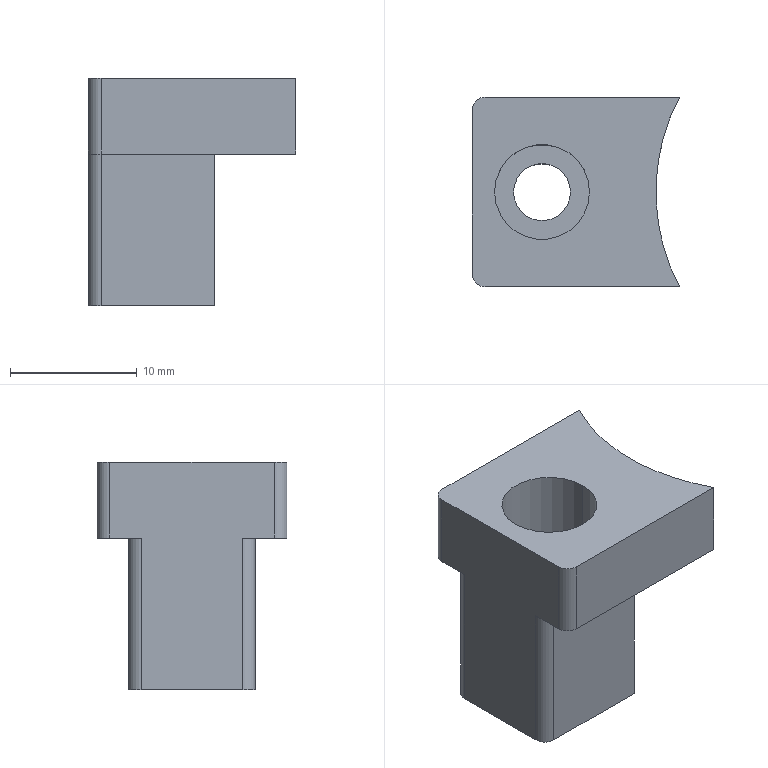Part | SolidWorks | features ICE 3, Fillet 2, Extrusion 1, HoleWzd 1, MirrorPattern 1 | 1 solid | 19 faces | box 16.367 x 15 x 18 mm | volume 2039 mm3 | plane 10 | cylinder 9 | commonest cylinder face diameters 2 x4 4.5 x2 7.5 x2 32 x1
STEP:
#1=CARTESIAN_POINT('',(-6.5,0.,10.));
#2=VERTEX_POINT('',#1);
#3=CARTESIAN_POINT('',(1.,0.,10.));
#4=VERTEX_POINT('',#3);
#5=CARTESIAN_POINT('',(-2.75,0.,10.));
#6=DIRECTION('',(0.,0.,1.));
#7=DIRECTION('',(1.,0.,0.));
#8=AXIS2_PLACEMENT_3D('',#5,#6,#7);
#9=CIRCLE('',#8,3.75);
#10=EDGE_CURVE('',#2,#4,#9,.T.);
#11=ORIENTED_EDGE('',*,*,#10,.F.);
#12=CARTESIAN_POINT('',(-6.5,0.,18.));
#13=VERTEX_POINT('',#12);
#14=CARTESIAN_POINT('',(-6.5,0.,18.));
#15=DIRECTION('',(0.,0.,1.));
#16=VECTOR('',#15,1000.);
#17=LINE('',#14,#16);
#18=EDGE_CURVE('',#2,#13,#17,.T.);
#19=ORIENTED_EDGE('',*,*,#18,.T.);
#20=CARTESIAN_POINT('',(1.,0.,18.));
#21=VERTEX_POINT('',#20);
#22=CARTESIAN_POINT('',(-2.75,0.,18.));
#23=DIRECTION('',(0.,0.,1.));
#24=DIRECTION('',(1.,0.,0.));
#25=AXIS2_PLACEMENT_3D('',#22,#23,#24);
#26=CIRCLE('',#25,3.75);
#27=EDGE_CURVE('',#13,#21,#26,.T.);
#28=ORIENTED_EDGE('',*,*,#27,.T.);
#29=CARTESIAN_POINT('',(1.,0.,18.));
#30=DIRECTION('',(0.,0.,1.));
#31=VECTOR('',#30,1000.);
#32=LINE('',#29,#31);
#33=EDGE_CURVE('',#4,#21,#32,.T.);
#34=ORIENTED_EDGE('',*,*,#33,.F.);
#35=EDGE_LOOP('',(#11,#19,#28,#34));
#36=FACE_OUTER_BOUND('',#35,.T.);
#37=CARTESIAN_POINT('',(-2.75,0.,18.));
#38=DIRECTION('',(0.,0.,1.));
#39=DIRECTION('',(1.,0.,0.));
#40=AXIS2_PLACEMENT_3D('',#37,#38,#39);
#41=CYLINDRICAL_SURFACE('',#40,3.75);
#42=ADVANCED_FACE('',(#36),#41,.F.);
#43=CARTESIAN_POINT('',(-5.,0.,0.));
#44=VERTEX_POINT('',#43);
#45=CARTESIAN_POINT('',(-0.5,0.,0.));
#46=VERTEX_POINT('',#45);
#47=CARTESIAN_POINT('',(-2.75,0.,0.));
#48=DIRECTION('',(0.,0.,1.));
#49=DIRECTION('',(1.,0.,0.));
#50=AXIS2_PLACEMENT_3D('',#47,#48,#49);
#51=CIRCLE('',#50,2.25);
#52=EDGE_CURVE('',#44,#46,#51,.T.);
#53=ORIENTED_EDGE('',*,*,#52,.F.);
#54=CARTESIAN_POINT('',(-5.,0.,10.));
#55=VERTEX_POINT('',#54);
#56=CARTESIAN_POINT('',(-5.,0.,18.));
#57=DIRECTION('',(0.,0.,1.));
#58=VECTOR('',#57,1000.);
#59=LINE('',#56,#58);
#60=EDGE_CURVE('',#44,#55,#59,.T.);
#61=ORIENTED_EDGE('',*,*,#60,.T.);
#62=CARTESIAN_POINT('',(-0.5,0.,10.));
#63=VERTEX_POINT('',#62);
#64=CARTESIAN_POINT('',(-2.75,0.,10.));
#65=DIRECTION('',(0.,0.,1.));
#66=DIRECTION('',(1.,0.,0.));
#67=AXIS2_PLACEMENT_3D('',#64,#65,#66);
#68=CIRCLE('',#67,2.25);
#69=EDGE_CURVE('',#55,#63,#68,.T.);
#70=ORIENTED_EDGE('',*,*,#69,.T.);
#71=CARTESIAN_POINT('',(-0.5,0.,18.));
#72=DIRECTION('',(0.,0.,1.));
#73=VECTOR('',#72,1000.);
#74=LINE('',#71,#73);
#75=EDGE_CURVE('',#46,#63,#74,.T.);
#76=ORIENTED_EDGE('',*,*,#75,.F.);
#77=EDGE_LOOP('',(#53,#61,#70,#76));
#78=FACE_OUTER_BOUND('',#77,.T.);
#79=CARTESIAN_POINT('',(-2.75,0.,18.));
#80=DIRECTION('',(0.,0.,1.));
#81=DIRECTION('',(1.,0.,0.));
#82=AXIS2_PLACEMENT_3D('',#79,#80,#81);
#83=CYLINDRICAL_SURFACE('',#82,2.25);
#84=ADVANCED_FACE('',(#78),#83,.F.);
#85=CARTESIAN_POINT('',(-7.25,7.5,12.));
#86=VERTEX_POINT('',#85);
#87=CARTESIAN_POINT('',(8.117,7.5,12.));
#88=VERTEX_POINT('',#87);
#89=CARTESIAN_POINT('',(1.75,7.5,12.));
#90=DIRECTION('',(1.,0.,0.));
#91=VECTOR('',#90,1000.);
#92=LINE('',#89,#91);
#93=EDGE_CURVE('',#86,#88,#92,.T.);
#94=ORIENTED_EDGE('',*,*,#93,.F.);
#95=CARTESIAN_POINT('',(-7.25,7.5,18.));
#96=VERTEX_POINT('',#95);
#97=CARTESIAN_POINT('',(-7.25,7.5,18.));
#98=DIRECTION('',(0.,0.,1.));
#99=VECTOR('',#98,1000.);
#100=LINE('',#97,#99);
#101=EDGE_CURVE('',#86,#96,#100,.T.);
#102=ORIENTED_EDGE('',*,*,#101,.T.);
#103=CARTESIAN_POINT('',(8.117,7.5,18.));
#104=VERTEX_POINT('',#103);
#105=CARTESIAN_POINT('',(-8.25,7.5,18.));
#106=DIRECTION('',(-1.,0.,0.));
#107=VECTOR('',#106,1000.);
#108=LINE('',#105,#107);
#109=EDGE_CURVE('',#104,#96,#108,.T.);
#110=ORIENTED_EDGE('',*,*,#109,.F.);
#111=CARTESIAN_POINT('',(8.117,7.5,0.));
#112=DIRECTION('',(0.,0.,-1.));
#113=VECTOR('',#112,1000.);
#114=LINE('',#111,#113);
#115=EDGE_CURVE('',#104,#88,#114,.T.);
#116=ORIENTED_EDGE('',*,*,#115,.T.);
#117=EDGE_LOOP('',(#94,#102,#110,#116));
#118=FACE_OUTER_BOUND('',#117,.T.);
#119=CARTESIAN_POINT('',(-8.25,7.5,18.));
#120=DIRECTION('',(0.,-1.,0.));
#121=DIRECTION('',(0.,0.,-1.));
#122=AXIS2_PLACEMENT_3D('',#119,#120,#121);
#123=PLANE('',#122);
#124=ADVANCED_FACE('',(#118),#123,.F.);
#125=CARTESIAN_POINT('',(-8.25,4.,12.));
#126=VERTEX_POINT('',#125);
#127=CARTESIAN_POINT('',(-8.25,6.5,12.));
#128=VERTEX_POINT('',#127);
#129=CARTESIAN_POINT('',(-8.25,5.,12.));
#130=DIRECTION('',(0.,1.,0.));
#131=VECTOR('',#130,1000.);
#132=LINE('',#129,#131);
#133=EDGE_CURVE('',#126,#128,#132,.T.);
#134=ORIENTED_EDGE('',*,*,#133,.F.);
#135=CARTESIAN_POINT('',(-8.25,4.,0.));
#136=VERTEX_POINT('',#135);
#137=CARTESIAN_POINT('',(-8.25,4.,18.));
#138=DIRECTION('',(0.,0.,-1.));
#139=VECTOR('',#138,1000.);
#140=LINE('',#137,#139);
#141=EDGE_CURVE('',#126,#136,#140,.T.);
#142=ORIENTED_EDGE('',*,*,#141,.T.);
#143=CARTESIAN_POINT('',(-8.25,-4.,0.));
#144=VERTEX_POINT('',#143);
#145=CARTESIAN_POINT('',(-8.25,7.5,0.));
#146=DIRECTION('',(0.,-1.,0.));
#147=VECTOR('',#146,1000.);
#148=LINE('',#145,#147);
#149=EDGE_CURVE('',#136,#144,#148,.T.);
#150=ORIENTED_EDGE('',*,*,#149,.T.);
#151=CARTESIAN_POINT('',(-8.25,-4.,12.));
#152=VERTEX_POINT('',#151);
#153=CARTESIAN_POINT('',(-8.25,-4.,18.));
#154=DIRECTION('',(0.,0.,1.));
#155=VECTOR('',#154,1000.);
#156=LINE('',#153,#155);
#157=EDGE_CURVE('',#144,#152,#156,.T.);
#158=ORIENTED_EDGE('',*,*,#157,.T.);
#159=CARTESIAN_POINT('',(-8.25,-6.5,12.));
#160=VERTEX_POINT('',#159);
#161=CARTESIAN_POINT('',(-8.25,-5.,12.));
#162=DIRECTION('',(0.,-1.,0.));
#163=VECTOR('',#162,1000.);
#164=LINE('',#161,#163);
#165=EDGE_CURVE('',#152,#160,#164,.T.);
#166=ORIENTED_EDGE('',*,*,#165,.T.);
#167=CARTESIAN_POINT('',(-8.25,-6.5,18.));
#168=VERTEX_POINT('',#167);
#169=CARTESIAN_POINT('',(-8.25,-6.5,18.));
#170=DIRECTION('',(0.,0.,1.));
#171=VECTOR('',#170,1000.);
#172=LINE('',#169,#171);
#173=EDGE_CURVE('',#160,#168,#172,.T.);
#174=ORIENTED_EDGE('',*,*,#173,.T.);
#175=CARTESIAN_POINT('',(-8.25,6.5,18.));
#176=VERTEX_POINT('',#175);
#177=CARTESIAN_POINT('',(-8.25,7.5,18.));
#178=DIRECTION('',(0.,-1.,0.));
#179=VECTOR('',#178,1000.);
#180=LINE('',#177,#179);
#181=EDGE_CURVE('',#176,#168,#180,.T.);
#182=ORIENTED_EDGE('',*,*,#181,.F.);
#183=CARTESIAN_POINT('',(-8.25,6.5,18.));
#184=DIRECTION('',(0.,0.,-1.));
#185=VECTOR('',#184,1000.);
#186=LINE('',#183,#185);
#187=EDGE_CURVE('',#176,#128,#186,.T.);
#188=ORIENTED_EDGE('',*,*,#187,.T.);
#189=EDGE_LOOP('',(#134,#142,#150,#158,#166,#174,#182,#188));
#190=FACE_OUTER_BOUND('',#189,.T.);
#191=CARTESIAN_POINT('',(-8.25,7.5,18.));
#192=DIRECTION('',(1.,0.,0.));
#193=DIRECTION('',(0.,1.,0.));
#194=AXIS2_PLACEMENT_3D('',#191,#192,#193);
#195=PLANE('',#194);
#196=ADVANCED_FACE('',(#190),#195,.F.);
#197=ORIENTED_EDGE('',*,*,#101,.F.);
#198=CARTESIAN_POINT('',(-7.25,6.5,12.));
#199=DIRECTION('',(0.,0.,1.));
#200=DIRECTION('',(-1.,0.,0.));
#201=AXIS2_PLACEMENT_3D('',#198,#199,#200);
#202=CIRCLE('',#201,1.);
#203=EDGE_CURVE('',#86,#128,#202,.T.);
#204=ORIENTED_EDGE('',*,*,#203,.T.);
#205=ORIENTED_EDGE('',*,*,#187,.F.);
#206=CARTESIAN_POINT('',(-7.25,6.5,18.));
#207=DIRECTION('',(0.,0.,1.));
#208=DIRECTION('',(1.,0.,0.));
#209=AXIS2_PLACEMENT_3D('',#206,#207,#208);
#210=CIRCLE('',#209,1.);
#211=EDGE_CURVE('',#96,#176,#210,.T.);
#212=ORIENTED_EDGE('',*,*,#211,.F.);
#213=EDGE_LOOP('',(#197,#204,#205,#212));
#214=FACE_OUTER_BOUND('',#213,.T.);
#215=CARTESIAN_POINT('',(-7.25,6.5,18.));
#216=DIRECTION('',(0.,0.,-1.));
#217=DIRECTION('',(-1.,0.,0.));
#218=AXIS2_PLACEMENT_3D('',#215,#216,#217);
#219=CYLINDRICAL_SURFACE('',#218,1.);
#220=ADVANCED_FACE('',(#214),#219,.T.);
#221=CARTESIAN_POINT('',(-7.25,-7.5,18.));
#222=VERTEX_POINT('',#221);
#223=CARTESIAN_POINT('',(-7.25,-7.5,12.));
#224=VERTEX_POINT('',#223);
#225=CARTESIAN_POINT('',(-7.25,-7.5,18.));
#226=DIRECTION('',(0.,0.,-1.));
#227=VECTOR('',#226,1000.);
#228=LINE('',#225,#227);
#229=EDGE_CURVE('',#222,#224,#228,.T.);
#230=ORIENTED_EDGE('',*,*,#229,.T.);
#231=CARTESIAN_POINT('',(8.117,-7.5,12.));
#232=VERTEX_POINT('',#231);
#233=CARTESIAN_POINT('',(1.75,-7.5,12.));
#234=DIRECTION('',(1.,0.,0.));
#235=VECTOR('',#234,1000.);
#236=LINE('',#233,#235);
#237=EDGE_CURVE('',#224,#232,#236,.T.);
#238=ORIENTED_EDGE('',*,*,#237,.T.);
#239=CARTESIAN_POINT('',(8.117,-7.5,18.));
#240=VERTEX_POINT('',#239);
#241=CARTESIAN_POINT('',(8.117,-7.5,0.));
#242=DIRECTION('',(0.,0.,1.));
#243=VECTOR('',#242,1000.);
#244=LINE('',#241,#243);
#245=EDGE_CURVE('',#232,#240,#244,.T.);
#246=ORIENTED_EDGE('',*,*,#245,.T.);
#247=CARTESIAN_POINT('',(-8.25,-7.5,18.));
#248=DIRECTION('',(1.,0.,0.));
#249=VECTOR('',#248,1000.);
#250=LINE('',#247,#249);
#251=EDGE_CURVE('',#222,#240,#250,.T.);
#252=ORIENTED_EDGE('',*,*,#251,.F.);
#253=EDGE_LOOP('',(#230,#238,#246,#252));
#254=FACE_OUTER_BOUND('',#253,.T.);
#255=CARTESIAN_POINT('',(-8.25,-7.5,18.));
#256=DIRECTION('',(0.,1.,0.));
#257=DIRECTION('',(0.,0.,1.));
#258=AXIS2_PLACEMENT_3D('',#255,#256,#257);
#259=PLANE('',#258);
#260=ADVANCED_FACE('',(#254),#259,.F.);
#261=CARTESIAN_POINT('',(22.25,0.,18.));
#262=DIRECTION('',(0.,0.,1.));
#263=DIRECTION('',(1.,0.,0.));
#264=AXIS2_PLACEMENT_3D('',#261,#262,#263);
#265=CIRCLE('',#264,16.);
#266=EDGE_CURVE('',#104,#240,#265,.T.);
#267=ORIENTED_EDGE('',*,*,#266,.F.);
#268=ORIENTED_EDGE('',*,*,#109,.T.);
#269=ORIENTED_EDGE('',*,*,#211,.T.);
#270=ORIENTED_EDGE('',*,*,#181,.T.);
#271=CARTESIAN_POINT('',(-7.25,-6.5,18.));
#272=DIRECTION('',(0.,0.,1.));
#273=DIRECTION('',(1.,0.,0.));
#274=AXIS2_PLACEMENT_3D('',#271,#272,#273);
#275=CIRCLE('',#274,1.);
#276=EDGE_CURVE('',#168,#222,#275,.T.);
#277=ORIENTED_EDGE('',*,*,#276,.T.);
#278=ORIENTED_EDGE('',*,*,#251,.T.);
#279=EDGE_LOOP('',(#267,#268,#269,#270,#277,#278));
#280=FACE_OUTER_BOUND('',#279,.T.);
#281=CARTESIAN_POINT('',(-2.75,0.,18.));
#282=DIRECTION('',(0.,0.,1.));
#283=DIRECTION('',(1.,0.,0.));
#284=AXIS2_PLACEMENT_3D('',#281,#282,#283);
#285=CIRCLE('',#284,3.75);
#286=EDGE_CURVE('',#21,#13,#285,.T.);
#287=ORIENTED_EDGE('',*,*,#286,.F.);
#288=ORIENTED_EDGE('',*,*,#27,.F.);
#289=EDGE_LOOP('',(#287,#288));
#290=FACE_BOUND('',#289,.T.);
#291=CARTESIAN_POINT('',(0.,0.,18.));
#292=DIRECTION('',(0.,0.,1.));
#293=DIRECTION('',(1.,0.,0.));
#294=AXIS2_PLACEMENT_3D('',#291,#292,#293);
#295=PLANE('',#294);
#296=ADVANCED_FACE('',(#280,#290),#295,.T.);
#297=CARTESIAN_POINT('',(-2.75,0.,0.));
#298=DIRECTION('',(0.,0.,1.));
#299=DIRECTION('',(1.,0.,0.));
#300=AXIS2_PLACEMENT_3D('',#297,#298,#299);
#301=CIRCLE('',#300,2.25);
#302=EDGE_CURVE('',#46,#44,#301,.T.);
#303=ORIENTED_EDGE('',*,*,#302,.T.);
#304=ORIENTED_EDGE('',*,*,#52,.T.);
#305=EDGE_LOOP('',(#303,#304));
#306=FACE_BOUND('',#305,.T.);
#307=ORIENTED_EDGE('',*,*,#149,.F.);
#308=CARTESIAN_POINT('',(-7.25,5.,0.));
#309=VERTEX_POINT('',#308);
#310=CARTESIAN_POINT('',(-7.25,4.,0.));
#311=DIRECTION('',(0.,0.,-1.));
#312=DIRECTION('',(1.,0.,0.));
#313=AXIS2_PLACEMENT_3D('',#310,#311,#312);
#314=CIRCLE('',#313,1.);
#315=EDGE_CURVE('',#136,#309,#314,.T.);
#316=ORIENTED_EDGE('',*,*,#315,.T.);
#317=CARTESIAN_POINT('',(1.75,5.,0.));
#318=VERTEX_POINT('',#317);
#319=CARTESIAN_POINT('',(-8.25,5.,0.));
#320=DIRECTION('',(1.,0.,0.));
#321=VECTOR('',#320,1000.);
#322=LINE('',#319,#321);
#323=EDGE_CURVE('',#309,#318,#322,.T.);
#324=ORIENTED_EDGE('',*,*,#323,.T.);
#325=CARTESIAN_POINT('',(1.75,-5.,0.));
#326=VERTEX_POINT('',#325);
#327=CARTESIAN_POINT('',(1.75,-7.5,0.));
#328=DIRECTION('',(0.,1.,0.));
#329=VECTOR('',#328,1000.);
#330=LINE('',#327,#329);
#331=EDGE_CURVE('',#326,#318,#330,.T.);
#332=ORIENTED_EDGE('',*,*,#331,.F.);
#333=CARTESIAN_POINT('',(-7.25,-5.,0.));
#334=VERTEX_POINT('',#333);
#335=CARTESIAN_POINT('',(-8.25,-5.,0.));
#336=DIRECTION('',(1.,0.,0.));
#337=VECTOR('',#336,1000.);
#338=LINE('',#335,#337);
#339=EDGE_CURVE('',#334,#326,#338,.T.);
#340=ORIENTED_EDGE('',*,*,#339,.F.);
#341=CARTESIAN_POINT('',(-7.25,-4.,0.));
#342=DIRECTION('',(0.,0.,-1.));
#343=DIRECTION('',(1.,0.,0.));
#344=AXIS2_PLACEMENT_3D('',#341,#342,#343);
#345=CIRCLE('',#344,1.);
#346=EDGE_CURVE('',#334,#144,#345,.T.);
#347=ORIENTED_EDGE('',*,*,#346,.T.);
#348=EDGE_LOOP('',(#307,#316,#324,#332,#340,#347));
#349=FACE_OUTER_BOUND('',#348,.T.);
#350=CARTESIAN_POINT('',(0.,0.,0.));
#351=DIRECTION('',(0.,0.,1.));
#352=DIRECTION('',(1.,0.,0.));
#353=AXIS2_PLACEMENT_3D('',#350,#351,#352);
#354=PLANE('',#353);
#355=ADVANCED_FACE('',(#306,#349),#354,.F.);
#356=CARTESIAN_POINT('',(-7.25,-6.5,12.));
#357=DIRECTION('',(0.,0.,-1.));
#358=DIRECTION('',(1.,0.,0.));
#359=AXIS2_PLACEMENT_3D('',#356,#357,#358);
#360=CIRCLE('',#359,1.);
#361=EDGE_CURVE('',#224,#160,#360,.T.);
#362=ORIENTED_EDGE('',*,*,#361,.F.);
#363=ORIENTED_EDGE('',*,*,#229,.F.);
#364=ORIENTED_EDGE('',*,*,#276,.F.);
#365=ORIENTED_EDGE('',*,*,#173,.F.);
#366=EDGE_LOOP('',(#362,#363,#364,#365));
#367=FACE_OUTER_BOUND('',#366,.T.);
#368=CARTESIAN_POINT('',(-7.25,-6.5,18.));
#369=DIRECTION('',(0.,0.,-1.));
#370=DIRECTION('',(-1.,0.,0.));
#371=AXIS2_PLACEMENT_3D('',#368,#369,#370);
#372=CYLINDRICAL_SURFACE('',#371,1.);
#373=ADVANCED_FACE('',(#367),#372,.T.);
#374=ORIENTED_EDGE('',*,*,#60,.F.);
#375=ORIENTED_EDGE('',*,*,#302,.F.);
#376=ORIENTED_EDGE('',*,*,#75,.T.);
#377=CARTESIAN_POINT('',(-2.75,0.,10.));
#378=DIRECTION('',(0.,0.,1.));
#379=DIRECTION('',(1.,0.,0.));
#380=AXIS2_PLACEMENT_3D('',#377,#378,#379);
#381=CIRCLE('',#380,2.25);
#382=EDGE_CURVE('',#63,#55,#381,.T.);
#383=ORIENTED_EDGE('',*,*,#382,.T.);
#384=EDGE_LOOP('',(#374,#375,#376,#383));
#385=FACE_OUTER_BOUND('',#384,.T.);
#386=CARTESIAN_POINT('',(-2.75,0.,18.));
#387=DIRECTION('',(0.,0.,1.));
#388=DIRECTION('',(1.,0.,0.));
#389=AXIS2_PLACEMENT_3D('',#386,#387,#388);
#390=CYLINDRICAL_SURFACE('',#389,2.25);
#391=ADVANCED_FACE('',(#385),#390,.F.);
#392=ORIENTED_EDGE('',*,*,#382,.F.);
#393=ORIENTED_EDGE('',*,*,#69,.F.);
#394=EDGE_LOOP('',(#392,#393));
#395=FACE_BOUND('',#394,.T.);
#396=CARTESIAN_POINT('',(-2.75,0.,10.));
#397=DIRECTION('',(0.,0.,1.));
#398=DIRECTION('',(1.,0.,0.));
#399=AXIS2_PLACEMENT_3D('',#396,#397,#398);
#400=CIRCLE('',#399,3.75);
#401=EDGE_CURVE('',#4,#2,#400,.T.);
#402=ORIENTED_EDGE('',*,*,#401,.T.);
#403=ORIENTED_EDGE('',*,*,#10,.T.);
#404=EDGE_LOOP('',(#402,#403));
#405=FACE_OUTER_BOUND('',#404,.T.);
#406=CARTESIAN_POINT('',(-0.5,0.,10.));
#407=DIRECTION('',(0.,0.,-1.));
#408=DIRECTION('',(-1.,0.,0.));
#409=AXIS2_PLACEMENT_3D('',#406,#407,#408);
#410=PLANE('',#409);
#411=ADVANCED_FACE('',(#395,#405),#410,.F.);
#412=ORIENTED_EDGE('',*,*,#18,.F.);
#413=ORIENTED_EDGE('',*,*,#401,.F.);
#414=ORIENTED_EDGE('',*,*,#33,.T.);
#415=ORIENTED_EDGE('',*,*,#286,.T.);
#416=EDGE_LOOP('',(#412,#413,#414,#415));
#417=FACE_OUTER_BOUND('',#416,.T.);
#418=CARTESIAN_POINT('',(-2.75,0.,18.));
#419=DIRECTION('',(0.,0.,1.));
#420=DIRECTION('',(1.,0.,0.));
#421=AXIS2_PLACEMENT_3D('',#418,#419,#420);
#422=CYLINDRICAL_SURFACE('',#421,3.75);
#423=ADVANCED_FACE('',(#417),#422,.F.);
#424=ORIENTED_EDGE('',*,*,#245,.F.);
#425=CARTESIAN_POINT('',(22.25,0.,12.));
#426=DIRECTION('',(0.,0.,-1.));
#427=DIRECTION('',(1.,0.,0.));
#428=AXIS2_PLACEMENT_3D('',#425,#426,#427);
#429=CIRCLE('',#428,16.);
#430=EDGE_CURVE('',#232,#88,#429,.T.);
#431=ORIENTED_EDGE('',*,*,#430,.T.);
#432=ORIENTED_EDGE('',*,*,#115,.F.);
#433=ORIENTED_EDGE('',*,*,#266,.T.);
#434=EDGE_LOOP('',(#424,#431,#432,#433));
#435=FACE_OUTER_BOUND('',#434,.T.);
#436=CARTESIAN_POINT('',(22.25,0.,0.));
#437=DIRECTION('',(0.,0.,1.));
#438=DIRECTION('',(1.,0.,0.));
#439=AXIS2_PLACEMENT_3D('',#436,#437,#438);
#440=CYLINDRICAL_SURFACE('',#439,16.);
#441=ADVANCED_FACE('',(#435),#440,.F.);
#442=ORIENTED_EDGE('',*,*,#237,.F.);
#443=ORIENTED_EDGE('',*,*,#361,.T.);
#444=ORIENTED_EDGE('',*,*,#165,.F.);
#445=CARTESIAN_POINT('',(-7.25,-5.,12.));
#446=VERTEX_POINT('',#445);
#447=CARTESIAN_POINT('',(-7.25,-4.,12.));
#448=DIRECTION('',(0.,0.,1.));
#449=DIRECTION('',(1.,0.,0.));
#450=AXIS2_PLACEMENT_3D('',#447,#448,#449);
#451=CIRCLE('',#450,1.);
#452=EDGE_CURVE('',#152,#446,#451,.T.);
#453=ORIENTED_EDGE('',*,*,#452,.T.);
#454=CARTESIAN_POINT('',(1.75,-5.,12.));
#455=VERTEX_POINT('',#454);
#456=CARTESIAN_POINT('',(-8.25,-5.,12.));
#457=DIRECTION('',(-1.,0.,0.));
#458=VECTOR('',#457,1000.);
#459=LINE('',#456,#458);
#460=EDGE_CURVE('',#455,#446,#459,.T.);
#461=ORIENTED_EDGE('',*,*,#460,.F.);
#462=CARTESIAN_POINT('',(1.75,5.,12.));
#463=VERTEX_POINT('',#462);
#464=CARTESIAN_POINT('',(1.75,-7.5,12.));
#465=DIRECTION('',(0.,1.,0.));
#466=VECTOR('',#465,1000.);
#467=LINE('',#464,#466);
#468=EDGE_CURVE('',#455,#463,#467,.T.);
#469=ORIENTED_EDGE('',*,*,#468,.T.);
#470=CARTESIAN_POINT('',(-7.25,5.,12.));
#471=VERTEX_POINT('',#470);
#472=CARTESIAN_POINT('',(-8.25,5.,12.));
#473=DIRECTION('',(-1.,0.,0.));
#474=VECTOR('',#473,1000.);
#475=LINE('',#472,#474);
#476=EDGE_CURVE('',#463,#471,#475,.T.);
#477=ORIENTED_EDGE('',*,*,#476,.T.);
#478=CARTESIAN_POINT('',(-7.25,4.,12.));
#479=DIRECTION('',(0.,0.,1.));
#480=DIRECTION('',(1.,0.,0.));
#481=AXIS2_PLACEMENT_3D('',#478,#479,#480);
#482=CIRCLE('',#481,1.);
#483=EDGE_CURVE('',#471,#126,#482,.T.);
#484=ORIENTED_EDGE('',*,*,#483,.T.);
#485=ORIENTED_EDGE('',*,*,#133,.T.);
#486=ORIENTED_EDGE('',*,*,#203,.F.);
#487=ORIENTED_EDGE('',*,*,#93,.T.);
#488=ORIENTED_EDGE('',*,*,#430,.F.);
#489=EDGE_LOOP('',(#442,#443,#444,#453,#461,#469,#477,#484,#485,#486,#487,#488));
#490=FACE_OUTER_BOUND('',#489,.T.);
#491=CARTESIAN_POINT('',(1.75,-7.5,12.));
#492=DIRECTION('',(0.,0.,1.));
#493=DIRECTION('',(1.,0.,0.));
#494=AXIS2_PLACEMENT_3D('',#491,#492,#493);
#495=PLANE('',#494);
#496=ADVANCED_FACE('',(#490),#495,.F.);
#497=ORIENTED_EDGE('',*,*,#331,.T.);
#498=CARTESIAN_POINT('',(1.75,5.,0.));
#499=DIRECTION('',(0.,0.,1.));
#500=VECTOR('',#499,1000.);
#501=LINE('',#498,#500);
#502=EDGE_CURVE('',#318,#463,#501,.T.);
#503=ORIENTED_EDGE('',*,*,#502,.T.);
#504=ORIENTED_EDGE('',*,*,#468,.F.);
#505=CARTESIAN_POINT('',(1.75,-5.,0.));
#506=DIRECTION('',(0.,0.,1.));
#507=VECTOR('',#506,1000.);
#508=LINE('',#505,#507);
#509=EDGE_CURVE('',#326,#455,#508,.T.);
#510=ORIENTED_EDGE('',*,*,#509,.F.);
#511=EDGE_LOOP('',(#497,#503,#504,#510));
#512=FACE_OUTER_BOUND('',#511,.T.);
#513=CARTESIAN_POINT('',(1.75,-7.5,0.));
#514=DIRECTION('',(-1.,0.,0.));
#515=DIRECTION('',(0.,0.,1.));
#516=AXIS2_PLACEMENT_3D('',#513,#514,#515);
#517=PLANE('',#516);
#518=ADVANCED_FACE('',(#512),#517,.F.);
#519=ORIENTED_EDGE('',*,*,#460,.T.);
#520=CARTESIAN_POINT('',(-7.25,-5.,0.));
#521=DIRECTION('',(0.,0.,-1.));
#522=VECTOR('',#521,1000.);
#523=LINE('',#520,#522);
#524=EDGE_CURVE('',#446,#334,#523,.T.);
#525=ORIENTED_EDGE('',*,*,#524,.T.);
#526=ORIENTED_EDGE('',*,*,#339,.T.);
#527=ORIENTED_EDGE('',*,*,#509,.T.);
#528=EDGE_LOOP('',(#519,#525,#526,#527));
#529=FACE_OUTER_BOUND('',#528,.T.);
#530=CARTESIAN_POINT('',(0.,-5.,0.));
#531=DIRECTION('',(0.,1.,0.));
#532=DIRECTION('',(0.,0.,1.));
#533=AXIS2_PLACEMENT_3D('',#530,#531,#532);
#534=PLANE('',#533);
#535=ADVANCED_FACE('',(#529),#534,.F.);
#536=ORIENTED_EDGE('',*,*,#323,.F.);
#537=CARTESIAN_POINT('',(-7.25,5.,0.));
#538=DIRECTION('',(0.,0.,1.));
#539=VECTOR('',#538,1000.);
#540=LINE('',#537,#539);
#541=EDGE_CURVE('',#309,#471,#540,.T.);
#542=ORIENTED_EDGE('',*,*,#541,.T.);
#543=ORIENTED_EDGE('',*,*,#476,.F.);
#544=ORIENTED_EDGE('',*,*,#502,.F.);
#545=EDGE_LOOP('',(#536,#542,#543,#544));
#546=FACE_OUTER_BOUND('',#545,.T.);
#547=CARTESIAN_POINT('',(0.,5.,0.));
#548=DIRECTION('',(0.,-1.,0.));
#549=DIRECTION('',(0.,0.,1.));
#550=AXIS2_PLACEMENT_3D('',#547,#548,#549);
#551=PLANE('',#550);
#552=ADVANCED_FACE('',(#546),#551,.F.);
#553=ORIENTED_EDGE('',*,*,#483,.F.);
#554=ORIENTED_EDGE('',*,*,#541,.F.);
#555=ORIENTED_EDGE('',*,*,#315,.F.);
#556=ORIENTED_EDGE('',*,*,#141,.F.);
#557=EDGE_LOOP('',(#553,#554,#555,#556));
#558=FACE_OUTER_BOUND('',#557,.T.);
#559=CARTESIAN_POINT('',(-7.25,4.,18.));
#560=DIRECTION('',(0.,0.,-1.));
#561=DIRECTION('',(-1.,0.,0.));
#562=AXIS2_PLACEMENT_3D('',#559,#560,#561);
#563=CYLINDRICAL_SURFACE('',#562,1.);
#564=ADVANCED_FACE('',(#558),#563,.T.);
#565=ORIENTED_EDGE('',*,*,#452,.F.);
#566=ORIENTED_EDGE('',*,*,#157,.F.);
#567=ORIENTED_EDGE('',*,*,#346,.F.);
#568=ORIENTED_EDGE('',*,*,#524,.F.);
#569=EDGE_LOOP('',(#565,#566,#567,#568));
#570=FACE_OUTER_BOUND('',#569,.T.);
#571=CARTESIAN_POINT('',(-7.25,-4.,0.));
#572=DIRECTION('',(0.,0.,-1.));
#573=DIRECTION('',(-1.,0.,0.));
#574=AXIS2_PLACEMENT_3D('',#571,#572,#573);
#575=CYLINDRICAL_SURFACE('',#574,1.);
#576=ADVANCED_FACE('',(#570),#575,.T.);
#577=CLOSED_SHELL('',(#42,#84,#124,#196,#220,#260,#296,#355,#373,#391,#411,#423,#441,#496,#518,#535,#552,#564,#576));
#578=MANIFOLD_SOLID_BREP('',#577);
#579=CARTESIAN_POINT('',(0.,0.,0.));
#580=DIRECTION('',(0.,0.,1.));
#581=DIRECTION('',(1.,0.,0.));
#582=AXIS2_PLACEMENT_3D('',#579,#580,#581);
#583=(LENGTH_UNIT()NAMED_UNIT(*)SI_UNIT(.MILLI.,.METRE.));
#584=UNCERTAINTY_MEASURE_WITH_UNIT(LENGTH_MEASURE(0.00001),#583,'','');
#585=(NAMED_UNIT(*)PLANE_ANGLE_UNIT()SI_UNIT($,.RADIAN.));
#586=(NAMED_UNIT(*)SI_UNIT($,.STERADIAN.)SOLID_ANGLE_UNIT());
#587=(GEOMETRIC_REPRESENTATION_CONTEXT(3)GLOBAL_UNCERTAINTY_ASSIGNED_CONTEXT((#584))GLOBAL_UNIT_ASSIGNED_CONTEXT((#583,#585,#586))REPRESENTATION_CONTEXT('',''));
#588=ADVANCED_BREP_SHAPE_REPRESENTATION('',(#578,#582),#587);